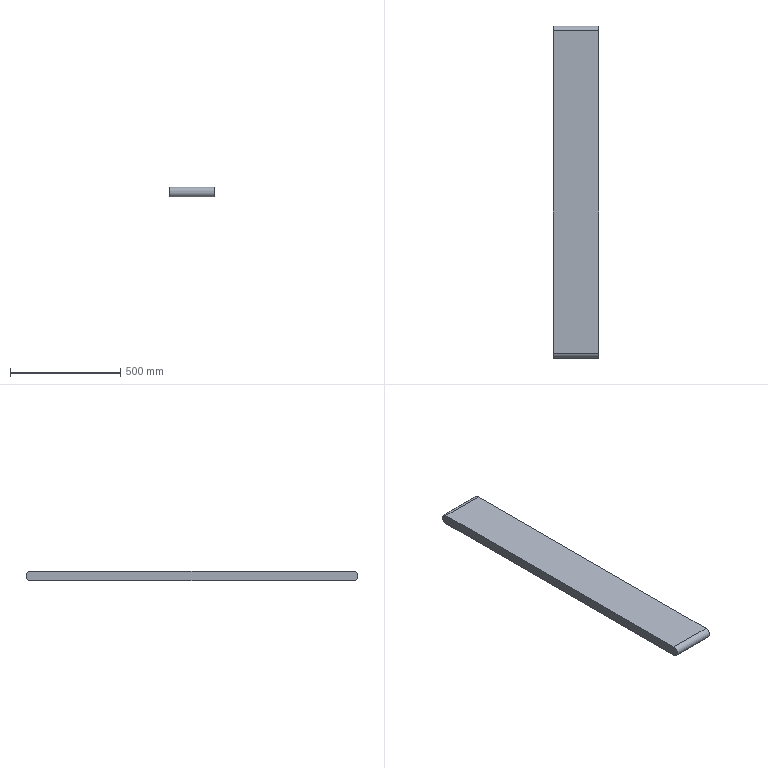Part | STEP file | lll_id4286_x_t | 1 solid | 6 faces | box 207 x 1505 x 45 mm | volume 13929119 mm3 | plane 4 | cylinder 2 | commonest cylinder face diameters 45 x2
STEP:
#1=CARTESIAN_POINT('',(4284.435,-690.,-380.));
#2=VERTEX_POINT('',#1);
#3=CARTESIAN_POINT('',(4284.435,770.,-380.));
#4=VERTEX_POINT('',#3);
#5=CARTESIAN_POINT('',(4284.435,0.,-380.));
#6=DIRECTION('',(0.,1.,0.));
#7=VECTOR('',#6,1.);
#8=LINE('',#5,#7);
#9=EDGE_CURVE('',#2,#4,#8,.T.);
#10=ORIENTED_EDGE('',*,*,#9,.F.);
#11=CARTESIAN_POINT('',(4077.435,-690.,-380.));
#12=VERTEX_POINT('',#11);
#13=CARTESIAN_POINT('',(4180.935,-690.,-380.));
#14=DIRECTION('',(-1.,0.,0.));
#15=VECTOR('',#14,1.);
#16=LINE('',#13,#15);
#17=EDGE_CURVE('',#2,#12,#16,.T.);
#18=ORIENTED_EDGE('',*,*,#17,.T.);
#19=CARTESIAN_POINT('',(4077.435,770.,-380.));
#20=VERTEX_POINT('',#19);
#21=CARTESIAN_POINT('',(4077.435,0.,-380.));
#22=DIRECTION('',(0.,1.,0.));
#23=VECTOR('',#22,1.);
#24=LINE('',#21,#23);
#25=EDGE_CURVE('',#12,#20,#24,.T.);
#26=ORIENTED_EDGE('',*,*,#25,.T.);
#27=CARTESIAN_POINT('',(4180.935,770.,-380.));
#28=DIRECTION('',(1.,0.,0.));
#29=VECTOR('',#28,1.);
#30=LINE('',#27,#29);
#31=EDGE_CURVE('',#20,#4,#30,.T.);
#32=ORIENTED_EDGE('',*,*,#31,.T.);
#33=EDGE_LOOP('',(#10,#18,#26,#32));
#34=FACE_OUTER_BOUND('',#33,.T.);
#35=CARTESIAN_POINT('',(4077.435,0.,-380.));
#36=DIRECTION('',(0.,0.,-1.));
#37=DIRECTION('',(0.,1.,0.));
#38=AXIS2_PLACEMENT_3D('',#35,#36,#37);
#39=PLANE('',#38);
#40=ADVANCED_FACE('',(#34),#39,.T.);
#41=CARTESIAN_POINT('',(4077.435,770.,-335.));
#42=VERTEX_POINT('',#41);
#43=CARTESIAN_POINT('',(4077.435,-690.,-335.));
#44=VERTEX_POINT('',#43);
#45=CARTESIAN_POINT('',(4077.435,0.,-335.));
#46=DIRECTION('',(0.,-1.,0.));
#47=VECTOR('',#46,1.);
#48=LINE('',#45,#47);
#49=EDGE_CURVE('',#42,#44,#48,.T.);
#50=ORIENTED_EDGE('',*,*,#49,.T.);
#51=CARTESIAN_POINT('',(4284.435,-690.,-335.));
#52=VERTEX_POINT('',#51);
#53=CARTESIAN_POINT('',(4180.935,-690.,-335.));
#54=DIRECTION('',(1.,0.,0.));
#55=VECTOR('',#54,1.);
#56=LINE('',#53,#55);
#57=EDGE_CURVE('',#44,#52,#56,.T.);
#58=ORIENTED_EDGE('',*,*,#57,.T.);
#59=CARTESIAN_POINT('',(4284.435,770.,-335.));
#60=VERTEX_POINT('',#59);
#61=CARTESIAN_POINT('',(4284.435,0.,-335.));
#62=DIRECTION('',(0.,-1.,0.));
#63=VECTOR('',#62,1.);
#64=LINE('',#61,#63);
#65=EDGE_CURVE('',#60,#52,#64,.T.);
#66=ORIENTED_EDGE('',*,*,#65,.F.);
#67=CARTESIAN_POINT('',(4180.935,770.,-335.));
#68=DIRECTION('',(-1.,0.,0.));
#69=VECTOR('',#68,1.);
#70=LINE('',#67,#69);
#71=EDGE_CURVE('',#60,#42,#70,.T.);
#72=ORIENTED_EDGE('',*,*,#71,.T.);
#73=EDGE_LOOP('',(#50,#58,#66,#72));
#74=FACE_OUTER_BOUND('',#73,.T.);
#75=CARTESIAN_POINT('',(4077.435,0.,-335.));
#76=DIRECTION('',(0.,0.,1.));
#77=DIRECTION('',(0.,-1.,0.));
#78=AXIS2_PLACEMENT_3D('',#75,#76,#77);
#79=PLANE('',#78);
#80=ADVANCED_FACE('',(#74),#79,.T.);
#81=ORIENTED_EDGE('',*,*,#65,.T.);
#82=CARTESIAN_POINT('',(4284.435,-690.,-357.5));
#83=DIRECTION('',(1.,0.,0.));
#84=DIRECTION('',(0.,0.,-1.));
#85=AXIS2_PLACEMENT_3D('',#82,#83,#84);
#86=CIRCLE('',#85,22.5);
#87=EDGE_CURVE('',#52,#2,#86,.T.);
#88=ORIENTED_EDGE('',*,*,#87,.T.);
#89=ORIENTED_EDGE('',*,*,#9,.T.);
#90=CARTESIAN_POINT('',(4284.435,770.,-357.5));
#91=DIRECTION('',(1.,0.,0.));
#92=DIRECTION('',(0.,0.,-1.));
#93=AXIS2_PLACEMENT_3D('',#90,#91,#92);
#94=CIRCLE('',#93,22.5);
#95=EDGE_CURVE('',#4,#60,#94,.T.);
#96=ORIENTED_EDGE('',*,*,#95,.T.);
#97=EDGE_LOOP('',(#81,#88,#89,#96));
#98=FACE_OUTER_BOUND('',#97,.T.);
#99=CARTESIAN_POINT('',(4284.435,0.,-405.));
#100=DIRECTION('',(1.,0.,0.));
#101=DIRECTION('',(0.,0.,-1.));
#102=AXIS2_PLACEMENT_3D('',#99,#100,#101);
#103=PLANE('',#102);
#104=ADVANCED_FACE('',(#98),#103,.T.);
#105=CARTESIAN_POINT('',(4077.435,-690.,-357.5));
#106=DIRECTION('',(-1.,0.,0.));
#107=DIRECTION('',(0.,0.,-1.));
#108=AXIS2_PLACEMENT_3D('',#105,#106,#107);
#109=CIRCLE('',#108,22.5);
#110=EDGE_CURVE('',#12,#44,#109,.T.);
#111=ORIENTED_EDGE('',*,*,#110,.T.);
#112=ORIENTED_EDGE('',*,*,#49,.F.);
#113=CARTESIAN_POINT('',(4077.435,770.,-357.5));
#114=DIRECTION('',(-1.,0.,0.));
#115=DIRECTION('',(0.,0.,-1.));
#116=AXIS2_PLACEMENT_3D('',#113,#114,#115);
#117=CIRCLE('',#116,22.5);
#118=EDGE_CURVE('',#42,#20,#117,.T.);
#119=ORIENTED_EDGE('',*,*,#118,.T.);
#120=ORIENTED_EDGE('',*,*,#25,.F.);
#121=EDGE_LOOP('',(#111,#112,#119,#120));
#122=FACE_OUTER_BOUND('',#121,.T.);
#123=CARTESIAN_POINT('',(4077.435,0.,-405.));
#124=DIRECTION('',(1.,0.,0.));
#125=DIRECTION('',(0.,0.,-1.));
#126=AXIS2_PLACEMENT_3D('',#123,#124,#125);
#127=PLANE('',#126);
#128=ADVANCED_FACE('',(#122),#127,.F.);
#129=ORIENTED_EDGE('',*,*,#95,.F.);
#130=ORIENTED_EDGE('',*,*,#31,.F.);
#131=ORIENTED_EDGE('',*,*,#118,.F.);
#132=ORIENTED_EDGE('',*,*,#71,.F.);
#133=EDGE_LOOP('',(#129,#130,#131,#132));
#134=FACE_OUTER_BOUND('',#133,.T.);
#135=CARTESIAN_POINT('',(4077.435,770.,-357.5));
#136=DIRECTION('',(1.,0.,0.));
#137=DIRECTION('',(0.,0.,-1.));
#138=AXIS2_PLACEMENT_3D('',#135,#136,#137);
#139=CYLINDRICAL_SURFACE('',#138,22.5);
#140=ADVANCED_FACE('',(#134),#139,.T.);
#141=ORIENTED_EDGE('',*,*,#87,.F.);
#142=ORIENTED_EDGE('',*,*,#57,.F.);
#143=ORIENTED_EDGE('',*,*,#110,.F.);
#144=ORIENTED_EDGE('',*,*,#17,.F.);
#145=EDGE_LOOP('',(#141,#142,#143,#144));
#146=FACE_OUTER_BOUND('',#145,.T.);
#147=CARTESIAN_POINT('',(4077.435,-690.,-357.5));
#148=DIRECTION('',(-1.,0.,0.));
#149=DIRECTION('',(0.,0.,1.));
#150=AXIS2_PLACEMENT_3D('',#147,#148,#149);
#151=CYLINDRICAL_SURFACE('',#150,22.5);
#152=ADVANCED_FACE('',(#146),#151,.T.);
#153=CLOSED_SHELL('',(#40,#80,#104,#128,#140,#152));
#154=MANIFOLD_SOLID_BREP('',#153);
#155=(LENGTH_UNIT()NAMED_UNIT(*)SI_UNIT(.MILLI.,.METRE.));
#156=UNCERTAINTY_MEASURE_WITH_UNIT(LENGTH_MEASURE(0.00002),#155,'','');
#157=(NAMED_UNIT(*)PLANE_ANGLE_UNIT()SI_UNIT($,.RADIAN.));
#158=PLANE_ANGLE_MEASURE_WITH_UNIT(PLANE_ANGLE_MEASURE(0.01745),#157);
#159=DIMENSIONAL_EXPONENTS(0.,0.,0.,0.,0.,0.,0.);
#160=(CONVERSION_BASED_UNIT('DEGREE',#158)NAMED_UNIT(#159)PLANE_ANGLE_UNIT());
#161=(NAMED_UNIT(*)SI_UNIT($,.STERADIAN.)SOLID_ANGLE_UNIT());
#162=(GEOMETRIC_REPRESENTATION_CONTEXT(3)GLOBAL_UNCERTAINTY_ASSIGNED_CONTEXT((#156))GLOBAL_UNIT_ASSIGNED_CONTEXT((#155,#160,#161))REPRESENTATION_CONTEXT('',''));
#163=ADVANCED_BREP_SHAPE_REPRESENTATION('',(#154),#162);